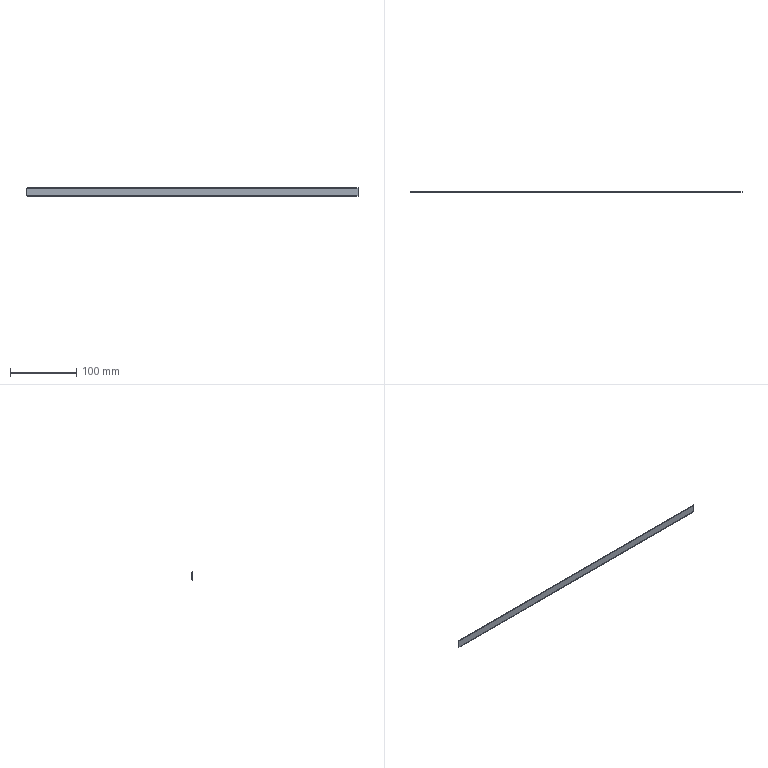Part | SolidWorks | features ICE 2, Extrusion 1 | 1 solid | 12 faces | box 503 x 0.6 x 13 mm | volume 3620 mm3 | plane 12
STEP:
#1=CARTESIAN_POINT('',(-250.,0.3,-5.5));
#2=VERTEX_POINT('',#1);
#3=CARTESIAN_POINT('',(-250.,-0.3,-5.5));
#4=VERTEX_POINT('',#3);
#5=CARTESIAN_POINT('',(-250.,0.3,-5.5));
#6=DIRECTION('',(0.,-1.,0.));
#7=VECTOR('',#6,1000.);
#8=LINE('',#5,#7);
#9=EDGE_CURVE('',#2,#4,#8,.T.);
#10=ORIENTED_EDGE('',*,*,#9,.F.);
#11=CARTESIAN_POINT('',(-250.,0.,-6.5));
#12=VERTEX_POINT('',#11);
#13=CARTESIAN_POINT('',(-250.,0.3,-5.5));
#14=DIRECTION('',(0.,-0.2873,-0.9578));
#15=VECTOR('',#14,1000.);
#16=LINE('',#13,#15);
#17=EDGE_CURVE('',#2,#12,#16,.T.);
#18=ORIENTED_EDGE('',*,*,#17,.T.);
#19=CARTESIAN_POINT('',(-250.,0.,-6.5));
#20=DIRECTION('',(0.,-0.2873,0.9578));
#21=VECTOR('',#20,1000.);
#22=LINE('',#19,#21);
#23=EDGE_CURVE('',#12,#4,#22,.T.);
#24=ORIENTED_EDGE('',*,*,#23,.T.);
#25=EDGE_LOOP('',(#10,#18,#24));
#26=FACE_OUTER_BOUND('',#25,.T.);
#27=CARTESIAN_POINT('',(-250.,0.3,0.));
#28=DIRECTION('',(-1.,0.,0.));
#29=DIRECTION('',(0.,0.,1.));
#30=AXIS2_PLACEMENT_3D('',#27,#28,#29);
#31=PLANE('',#30);
#32=ADVANCED_FACE('',(#26),#31,.T.);
#33=CARTESIAN_POINT('',(250.,-0.3,5.5));
#34=VERTEX_POINT('',#33);
#35=CARTESIAN_POINT('',(250.,-0.3,-5.5));
#36=VERTEX_POINT('',#35);
#37=CARTESIAN_POINT('',(250.,-0.3,0.));
#38=DIRECTION('',(0.,0.,-1.));
#39=VECTOR('',#38,1000.);
#40=LINE('',#37,#39);
#41=EDGE_CURVE('',#34,#36,#40,.T.);
#42=ORIENTED_EDGE('',*,*,#41,.T.);
#43=CARTESIAN_POINT('',(250.,0.,-6.5));
#44=VERTEX_POINT('',#43);
#45=CARTESIAN_POINT('',(250.,0.,-6.5));
#46=DIRECTION('',(0.,-0.2873,0.9578));
#47=VECTOR('',#46,1000.);
#48=LINE('',#45,#47);
#49=EDGE_CURVE('',#44,#36,#48,.T.);
#50=ORIENTED_EDGE('',*,*,#49,.F.);
#51=CARTESIAN_POINT('',(250.,0.3,-5.5));
#52=VERTEX_POINT('',#51);
#53=CARTESIAN_POINT('',(250.,0.3,-5.5));
#54=DIRECTION('',(0.,-0.2873,-0.9578));
#55=VECTOR('',#54,1000.);
#56=LINE('',#53,#55);
#57=EDGE_CURVE('',#52,#44,#56,.T.);
#58=ORIENTED_EDGE('',*,*,#57,.F.);
#59=CARTESIAN_POINT('',(250.,0.3,5.5));
#60=VERTEX_POINT('',#59);
#61=CARTESIAN_POINT('',(250.,0.3,0.));
#62=DIRECTION('',(0.,0.,-1.));
#63=VECTOR('',#62,1000.);
#64=LINE('',#61,#63);
#65=EDGE_CURVE('',#60,#52,#64,.T.);
#66=ORIENTED_EDGE('',*,*,#65,.F.);
#67=CARTESIAN_POINT('',(250.,0.,6.5));
#68=VERTEX_POINT('',#67);
#69=CARTESIAN_POINT('',(250.,0.3,5.5));
#70=DIRECTION('',(0.,0.2873,-0.9578));
#71=VECTOR('',#70,1000.);
#72=LINE('',#69,#71);
#73=EDGE_CURVE('',#68,#60,#72,.T.);
#74=ORIENTED_EDGE('',*,*,#73,.F.);
#75=CARTESIAN_POINT('',(250.,0.,6.5));
#76=DIRECTION('',(0.,0.2873,0.9578));
#77=VECTOR('',#76,1000.);
#78=LINE('',#75,#77);
#79=EDGE_CURVE('',#34,#68,#78,.T.);
#80=ORIENTED_EDGE('',*,*,#79,.F.);
#81=EDGE_LOOP('',(#42,#50,#58,#66,#74,#80));
#82=FACE_OUTER_BOUND('',#81,.T.);
#83=CARTESIAN_POINT('',(250.,0.3,0.));
#84=DIRECTION('',(-1.,0.,0.));
#85=DIRECTION('',(0.,0.,1.));
#86=AXIS2_PLACEMENT_3D('',#83,#84,#85);
#87=PLANE('',#86);
#88=ADVANCED_FACE('',(#82),#87,.F.);
#89=CARTESIAN_POINT('',(-250.,-0.3,5.5));
#90=VERTEX_POINT('',#89);
#91=CARTESIAN_POINT('',(-250.,0.3,5.5));
#92=VERTEX_POINT('',#91);
#93=CARTESIAN_POINT('',(-250.,0.3,5.5));
#94=DIRECTION('',(0.,1.,0.));
#95=VECTOR('',#94,1000.);
#96=LINE('',#93,#95);
#97=EDGE_CURVE('',#90,#92,#96,.T.);
#98=ORIENTED_EDGE('',*,*,#97,.F.);
#99=CARTESIAN_POINT('',(-250.,0.,6.5));
#100=VERTEX_POINT('',#99);
#101=CARTESIAN_POINT('',(-250.,0.,6.5));
#102=DIRECTION('',(0.,0.2873,0.9578));
#103=VECTOR('',#102,1000.);
#104=LINE('',#101,#103);
#105=EDGE_CURVE('',#90,#100,#104,.T.);
#106=ORIENTED_EDGE('',*,*,#105,.T.);
#107=CARTESIAN_POINT('',(-250.,0.3,5.5));
#108=DIRECTION('',(0.,0.2873,-0.9578));
#109=VECTOR('',#108,1000.);
#110=LINE('',#107,#109);
#111=EDGE_CURVE('',#100,#92,#110,.T.);
#112=ORIENTED_EDGE('',*,*,#111,.T.);
#113=EDGE_LOOP('',(#98,#106,#112));
#114=FACE_OUTER_BOUND('',#113,.T.);
#115=CARTESIAN_POINT('',(-250.,0.3,0.));
#116=DIRECTION('',(-1.,0.,0.));
#117=DIRECTION('',(0.,0.,1.));
#118=AXIS2_PLACEMENT_3D('',#115,#116,#117);
#119=PLANE('',#118);
#120=ADVANCED_FACE('',(#114),#119,.T.);
#121=CARTESIAN_POINT('',(-250.,0.3,-5.5));
#122=DIRECTION('',(1.,0.,0.));
#123=VECTOR('',#122,1000.);
#124=LINE('',#121,#123);
#125=EDGE_CURVE('',#2,#52,#124,.T.);
#126=ORIENTED_EDGE('',*,*,#125,.F.);
#127=CARTESIAN_POINT('',(-253.,0.3,-5.5));
#128=VERTEX_POINT('',#127);
#129=CARTESIAN_POINT('',(-253.,0.3,-5.5));
#130=DIRECTION('',(1.,0.,0.));
#131=VECTOR('',#130,1000.);
#132=LINE('',#129,#131);
#133=EDGE_CURVE('',#128,#2,#132,.T.);
#134=ORIENTED_EDGE('',*,*,#133,.F.);
#135=CARTESIAN_POINT('',(-253.,0.3,5.5));
#136=VERTEX_POINT('',#135);
#137=CARTESIAN_POINT('',(-253.,0.3,-5.5));
#138=DIRECTION('',(0.,0.,-1.));
#139=VECTOR('',#138,1000.);
#140=LINE('',#137,#139);
#141=EDGE_CURVE('',#136,#128,#140,.T.);
#142=ORIENTED_EDGE('',*,*,#141,.F.);
#143=CARTESIAN_POINT('',(-253.,0.3,5.5));
#144=DIRECTION('',(1.,0.,0.));
#145=VECTOR('',#144,1000.);
#146=LINE('',#143,#145);
#147=EDGE_CURVE('',#136,#92,#146,.T.);
#148=ORIENTED_EDGE('',*,*,#147,.T.);
#149=CARTESIAN_POINT('',(-250.,0.3,5.5));
#150=DIRECTION('',(1.,0.,0.));
#151=VECTOR('',#150,1000.);
#152=LINE('',#149,#151);
#153=EDGE_CURVE('',#92,#60,#152,.T.);
#154=ORIENTED_EDGE('',*,*,#153,.T.);
#155=ORIENTED_EDGE('',*,*,#65,.T.);
#156=EDGE_LOOP('',(#126,#134,#142,#148,#154,#155));
#157=FACE_OUTER_BOUND('',#156,.T.);
#158=CARTESIAN_POINT('',(0.,0.3,0.));
#159=DIRECTION('',(0.,1.,0.));
#160=DIRECTION('',(0.,0.,1.));
#161=AXIS2_PLACEMENT_3D('',#158,#159,#160);
#162=PLANE('',#161);
#163=ADVANCED_FACE('',(#157),#162,.T.);
#164=CARTESIAN_POINT('',(-250.,-0.3,5.5));
#165=DIRECTION('',(1.,0.,0.));
#166=VECTOR('',#165,1000.);
#167=LINE('',#164,#166);
#168=EDGE_CURVE('',#90,#34,#167,.T.);
#169=ORIENTED_EDGE('',*,*,#168,.F.);
#170=CARTESIAN_POINT('',(-253.,-0.3,5.5));
#171=VERTEX_POINT('',#170);
#172=CARTESIAN_POINT('',(-253.,-0.3,5.5));
#173=DIRECTION('',(1.,0.,0.));
#174=VECTOR('',#173,1000.);
#175=LINE('',#172,#174);
#176=EDGE_CURVE('',#171,#90,#175,.T.);
#177=ORIENTED_EDGE('',*,*,#176,.F.);
#178=CARTESIAN_POINT('',(-253.,-0.3,-5.5));
#179=VERTEX_POINT('',#178);
#180=CARTESIAN_POINT('',(-253.,-0.3,-5.5));
#181=DIRECTION('',(0.,0.,1.));
#182=VECTOR('',#181,1000.);
#183=LINE('',#180,#182);
#184=EDGE_CURVE('',#179,#171,#183,.T.);
#185=ORIENTED_EDGE('',*,*,#184,.F.);
#186=CARTESIAN_POINT('',(-253.,-0.3,-5.5));
#187=DIRECTION('',(1.,0.,0.));
#188=VECTOR('',#187,1000.);
#189=LINE('',#186,#188);
#190=EDGE_CURVE('',#179,#4,#189,.T.);
#191=ORIENTED_EDGE('',*,*,#190,.T.);
#192=CARTESIAN_POINT('',(-250.,-0.3,-5.5));
#193=DIRECTION('',(1.,0.,0.));
#194=VECTOR('',#193,1000.);
#195=LINE('',#192,#194);
#196=EDGE_CURVE('',#4,#36,#195,.T.);
#197=ORIENTED_EDGE('',*,*,#196,.T.);
#198=ORIENTED_EDGE('',*,*,#41,.F.);
#199=EDGE_LOOP('',(#169,#177,#185,#191,#197,#198));
#200=FACE_OUTER_BOUND('',#199,.T.);
#201=CARTESIAN_POINT('',(0.,-0.3,0.));
#202=DIRECTION('',(0.,1.,0.));
#203=DIRECTION('',(0.,0.,1.));
#204=AXIS2_PLACEMENT_3D('',#201,#202,#203);
#205=PLANE('',#204);
#206=ADVANCED_FACE('',(#200),#205,.F.);
#207=ORIENTED_EDGE('',*,*,#153,.F.);
#208=ORIENTED_EDGE('',*,*,#111,.F.);
#209=CARTESIAN_POINT('',(-250.,0.,6.5));
#210=DIRECTION('',(1.,0.,0.));
#211=VECTOR('',#210,1000.);
#212=LINE('',#209,#211);
#213=EDGE_CURVE('',#100,#68,#212,.T.);
#214=ORIENTED_EDGE('',*,*,#213,.T.);
#215=ORIENTED_EDGE('',*,*,#73,.T.);
#216=EDGE_LOOP('',(#207,#208,#214,#215));
#217=FACE_OUTER_BOUND('',#216,.T.);
#218=CARTESIAN_POINT('',(-250.,0.3,5.5));
#219=DIRECTION('',(0.,-0.9578,-0.2873));
#220=DIRECTION('',(0.,0.2873,-0.9578));
#221=AXIS2_PLACEMENT_3D('',#218,#219,#220);
#222=PLANE('',#221);
#223=ADVANCED_FACE('',(#217),#222,.F.);
#224=ORIENTED_EDGE('',*,*,#213,.F.);
#225=ORIENTED_EDGE('',*,*,#105,.F.);
#226=ORIENTED_EDGE('',*,*,#168,.T.);
#227=ORIENTED_EDGE('',*,*,#79,.T.);
#228=EDGE_LOOP('',(#224,#225,#226,#227));
#229=FACE_OUTER_BOUND('',#228,.T.);
#230=CARTESIAN_POINT('',(-250.,0.,6.5));
#231=DIRECTION('',(0.,0.9578,-0.2873));
#232=DIRECTION('',(0.,0.2873,0.9578));
#233=AXIS2_PLACEMENT_3D('',#230,#231,#232);
#234=PLANE('',#233);
#235=ADVANCED_FACE('',(#229),#234,.F.);
#236=ORIENTED_EDGE('',*,*,#196,.F.);
#237=ORIENTED_EDGE('',*,*,#23,.F.);
#238=CARTESIAN_POINT('',(-250.,0.,-6.5));
#239=DIRECTION('',(1.,0.,0.));
#240=VECTOR('',#239,1000.);
#241=LINE('',#238,#240);
#242=EDGE_CURVE('',#12,#44,#241,.T.);
#243=ORIENTED_EDGE('',*,*,#242,.T.);
#244=ORIENTED_EDGE('',*,*,#49,.T.);
#245=EDGE_LOOP('',(#236,#237,#243,#244));
#246=FACE_OUTER_BOUND('',#245,.T.);
#247=CARTESIAN_POINT('',(-250.,0.,-6.5));
#248=DIRECTION('',(0.,0.9578,0.2873));
#249=DIRECTION('',(0.,-0.2873,0.9578));
#250=AXIS2_PLACEMENT_3D('',#247,#248,#249);
#251=PLANE('',#250);
#252=ADVANCED_FACE('',(#246),#251,.F.);
#253=ORIENTED_EDGE('',*,*,#242,.F.);
#254=ORIENTED_EDGE('',*,*,#17,.F.);
#255=ORIENTED_EDGE('',*,*,#125,.T.);
#256=ORIENTED_EDGE('',*,*,#57,.T.);
#257=EDGE_LOOP('',(#253,#254,#255,#256));
#258=FACE_OUTER_BOUND('',#257,.T.);
#259=CARTESIAN_POINT('',(-250.,0.3,-5.5));
#260=DIRECTION('',(0.,-0.9578,0.2873));
#261=DIRECTION('',(0.,-0.2873,-0.9578));
#262=AXIS2_PLACEMENT_3D('',#259,#260,#261);
#263=PLANE('',#262);
#264=ADVANCED_FACE('',(#258),#263,.F.);
#265=ORIENTED_EDGE('',*,*,#9,.T.);
#266=ORIENTED_EDGE('',*,*,#190,.F.);
#267=CARTESIAN_POINT('',(-253.,0.3,-5.5));
#268=DIRECTION('',(0.,-1.,0.));
#269=VECTOR('',#268,1000.);
#270=LINE('',#267,#269);
#271=EDGE_CURVE('',#128,#179,#270,.T.);
#272=ORIENTED_EDGE('',*,*,#271,.F.);
#273=ORIENTED_EDGE('',*,*,#133,.T.);
#274=EDGE_LOOP('',(#265,#266,#272,#273));
#275=FACE_OUTER_BOUND('',#274,.T.);
#276=CARTESIAN_POINT('',(-253.,0.3,-5.5));
#277=DIRECTION('',(0.,0.,1.));
#278=DIRECTION('',(1.,0.,0.));
#279=AXIS2_PLACEMENT_3D('',#276,#277,#278);
#280=PLANE('',#279);
#281=ADVANCED_FACE('',(#275),#280,.F.);
#282=ORIENTED_EDGE('',*,*,#97,.T.);
#283=ORIENTED_EDGE('',*,*,#147,.F.);
#284=CARTESIAN_POINT('',(-253.,0.3,5.5));
#285=DIRECTION('',(0.,1.,0.));
#286=VECTOR('',#285,1000.);
#287=LINE('',#284,#286);
#288=EDGE_CURVE('',#171,#136,#287,.T.);
#289=ORIENTED_EDGE('',*,*,#288,.F.);
#290=ORIENTED_EDGE('',*,*,#176,.T.);
#291=EDGE_LOOP('',(#282,#283,#289,#290));
#292=FACE_OUTER_BOUND('',#291,.T.);
#293=CARTESIAN_POINT('',(-253.,0.3,5.5));
#294=DIRECTION('',(0.,0.,-1.));
#295=DIRECTION('',(-1.,0.,0.));
#296=AXIS2_PLACEMENT_3D('',#293,#294,#295);
#297=PLANE('',#296);
#298=ADVANCED_FACE('',(#292),#297,.F.);
#299=ORIENTED_EDGE('',*,*,#271,.T.);
#300=ORIENTED_EDGE('',*,*,#184,.T.);
#301=ORIENTED_EDGE('',*,*,#288,.T.);
#302=ORIENTED_EDGE('',*,*,#141,.T.);
#303=EDGE_LOOP('',(#299,#300,#301,#302));
#304=FACE_OUTER_BOUND('',#303,.T.);
#305=CARTESIAN_POINT('',(-253.,0.,0.));
#306=DIRECTION('',(-1.,0.,0.));
#307=DIRECTION('',(0.,0.,1.));
#308=AXIS2_PLACEMENT_3D('',#305,#306,#307);
#309=PLANE('',#308);
#310=ADVANCED_FACE('',(#304),#309,.T.);
#311=CLOSED_SHELL('',(#32,#88,#120,#163,#206,#223,#235,#252,#264,#281,#298,#310));
#312=MANIFOLD_SOLID_BREP('',#311);
#313=CARTESIAN_POINT('',(0.,0.,0.));
#314=DIRECTION('',(0.,0.,1.));
#315=DIRECTION('',(1.,0.,0.));
#316=AXIS2_PLACEMENT_3D('',#313,#314,#315);
#317=(LENGTH_UNIT()NAMED_UNIT(*)SI_UNIT(.MILLI.,.METRE.));
#318=UNCERTAINTY_MEASURE_WITH_UNIT(LENGTH_MEASURE(0.00001),#317,'','');
#319=(NAMED_UNIT(*)PLANE_ANGLE_UNIT()SI_UNIT($,.RADIAN.));
#320=(NAMED_UNIT(*)SI_UNIT($,.STERADIAN.)SOLID_ANGLE_UNIT());
#321=(GEOMETRIC_REPRESENTATION_CONTEXT(3)GLOBAL_UNCERTAINTY_ASSIGNED_CONTEXT((#318))GLOBAL_UNIT_ASSIGNED_CONTEXT((#317,#319,#320))REPRESENTATION_CONTEXT('',''));
#322=ADVANCED_BREP_SHAPE_REPRESENTATION('',(#312,#316),#321);